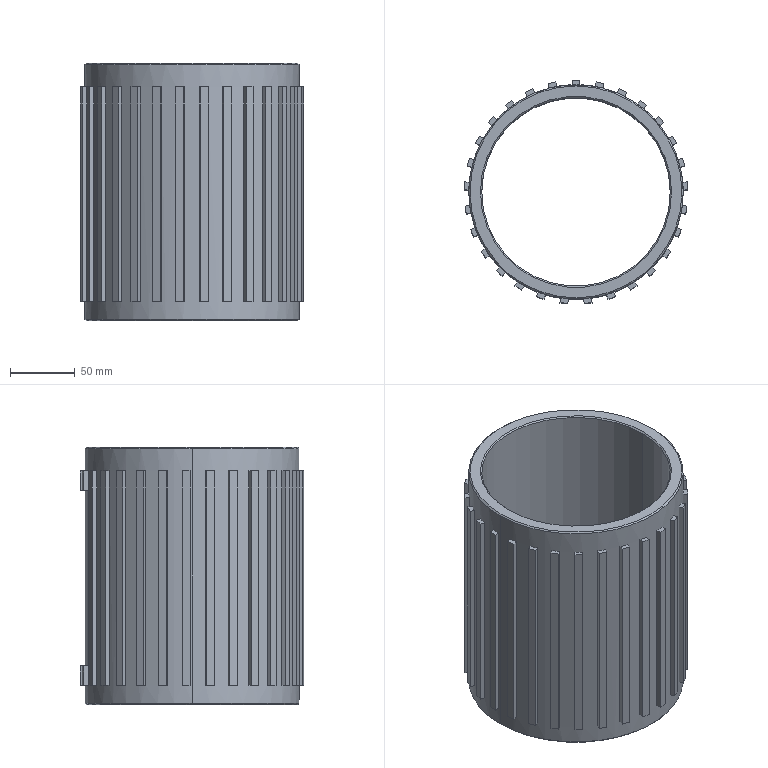Part | SolidWorks | features BaseBody 1 | 1 solid | 185 faces | box 172.079 x 171.827 x 198 mm | volume 1054388 mm3 | plane 173 | cone 8 | cylinder 4 | commonest cylinder face diameters 145 x2 165 x2